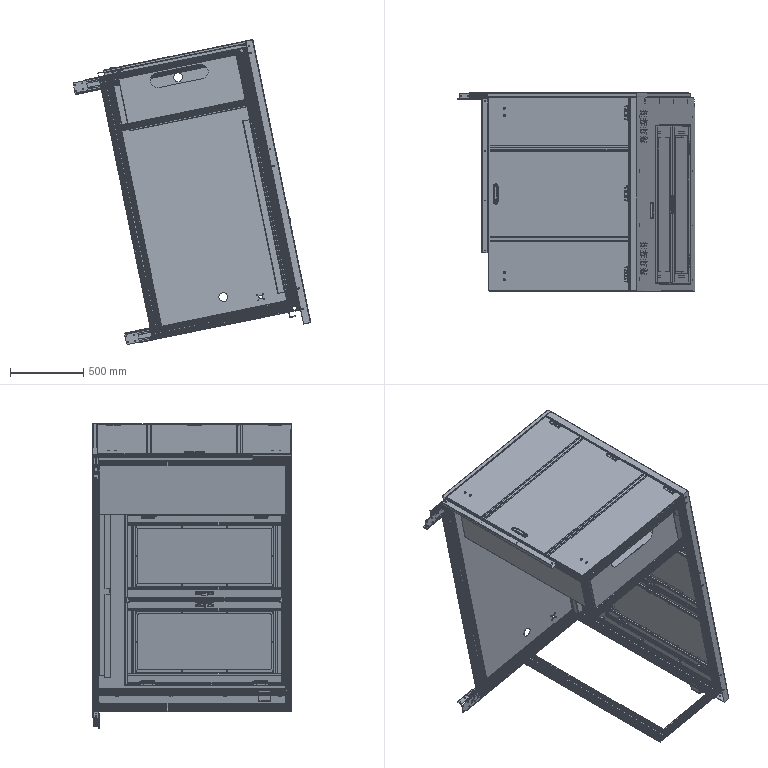Part | NX | features BREP 43 | 86 solids | 7754 faces | volume 38224083 mm3 | plane 4000 | cylinder 3427 | cone 173 | spline 92 | torus 62 | commonest cylinder face diameters 1 x758 0.4 x627 4 x312 7 x301 6 x261 3 x209